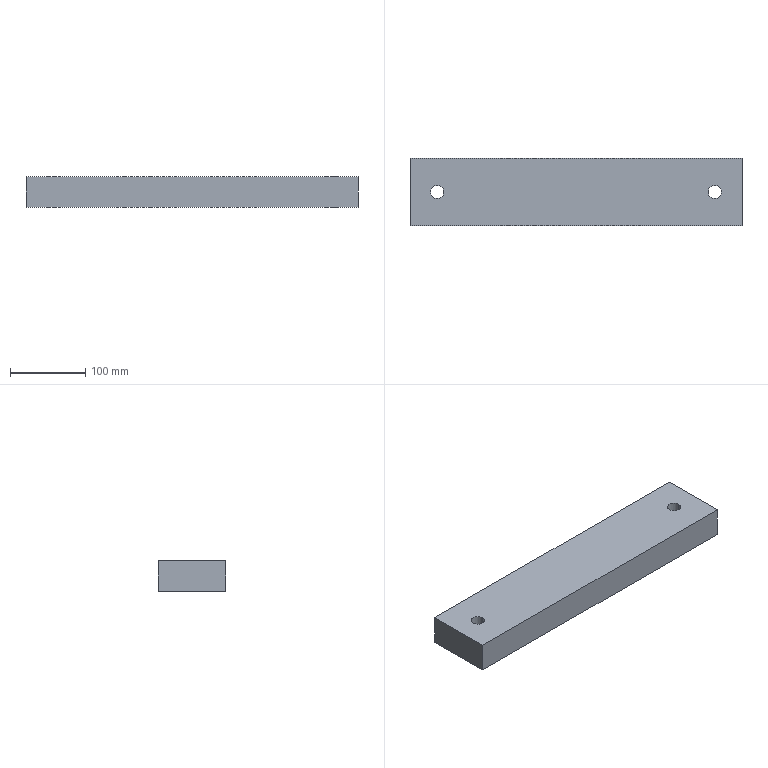Part | SolidWorks | features Extrusion 1, HoleWzd 1 | 1 solid | 10 faces | box 440 x 90 x 40 mm | volume 1564758 mm3 | plane 6 | cylinder 4 | commonest cylinder face diameters 17.5 x4
STEP:
#1=CARTESIAN_POINT('',(27.25,45.,0.));
#2=VERTEX_POINT('',#1);
#3=CARTESIAN_POINT('',(44.75,45.,0.));
#4=VERTEX_POINT('',#3);
#5=CARTESIAN_POINT('',(36.,45.,0.));
#6=DIRECTION('',(0.,0.,1.));
#7=DIRECTION('',(1.,0.,0.));
#8=AXIS2_PLACEMENT_3D('',#5,#6,#7);
#9=CIRCLE('',#8,8.75);
#10=EDGE_CURVE('',#2,#4,#9,.T.);
#11=ORIENTED_EDGE('',*,*,#10,.F.);
#12=CARTESIAN_POINT('',(27.25,45.,40.));
#13=VERTEX_POINT('',#12);
#14=CARTESIAN_POINT('',(27.25,45.,40.));
#15=DIRECTION('',(0.,0.,1.));
#16=VECTOR('',#15,1000.);
#17=LINE('',#14,#16);
#18=EDGE_CURVE('',#2,#13,#17,.T.);
#19=ORIENTED_EDGE('',*,*,#18,.T.);
#20=CARTESIAN_POINT('',(44.75,45.,40.));
#21=VERTEX_POINT('',#20);
#22=CARTESIAN_POINT('',(36.,45.,40.));
#23=DIRECTION('',(0.,0.,1.));
#24=DIRECTION('',(1.,0.,0.));
#25=AXIS2_PLACEMENT_3D('',#22,#23,#24);
#26=CIRCLE('',#25,8.75);
#27=EDGE_CURVE('',#13,#21,#26,.T.);
#28=ORIENTED_EDGE('',*,*,#27,.T.);
#29=CARTESIAN_POINT('',(44.75,45.,40.));
#30=DIRECTION('',(0.,0.,1.));
#31=VECTOR('',#30,1000.);
#32=LINE('',#29,#31);
#33=EDGE_CURVE('',#4,#21,#32,.T.);
#34=ORIENTED_EDGE('',*,*,#33,.F.);
#35=EDGE_LOOP('',(#11,#19,#28,#34));
#36=FACE_OUTER_BOUND('',#35,.T.);
#37=CARTESIAN_POINT('',(36.,45.,40.));
#38=DIRECTION('',(0.,0.,1.));
#39=DIRECTION('',(1.,0.,0.));
#40=AXIS2_PLACEMENT_3D('',#37,#38,#39);
#41=CYLINDRICAL_SURFACE('',#40,8.75);
#42=ADVANCED_FACE('',(#36),#41,.F.);
#43=CARTESIAN_POINT('',(395.25,45.,0.));
#44=VERTEX_POINT('',#43);
#45=CARTESIAN_POINT('',(412.75,45.,0.));
#46=VERTEX_POINT('',#45);
#47=CARTESIAN_POINT('',(404.,45.,0.));
#48=DIRECTION('',(0.,0.,1.));
#49=DIRECTION('',(1.,0.,0.));
#50=AXIS2_PLACEMENT_3D('',#47,#48,#49);
#51=CIRCLE('',#50,8.75);
#52=EDGE_CURVE('',#44,#46,#51,.T.);
#53=ORIENTED_EDGE('',*,*,#52,.F.);
#54=CARTESIAN_POINT('',(395.25,45.,40.));
#55=VERTEX_POINT('',#54);
#56=CARTESIAN_POINT('',(395.25,45.,40.));
#57=DIRECTION('',(0.,0.,1.));
#58=VECTOR('',#57,1000.);
#59=LINE('',#56,#58);
#60=EDGE_CURVE('',#44,#55,#59,.T.);
#61=ORIENTED_EDGE('',*,*,#60,.T.);
#62=CARTESIAN_POINT('',(412.75,45.,40.));
#63=VERTEX_POINT('',#62);
#64=CARTESIAN_POINT('',(404.,45.,40.));
#65=DIRECTION('',(0.,0.,1.));
#66=DIRECTION('',(1.,0.,0.));
#67=AXIS2_PLACEMENT_3D('',#64,#65,#66);
#68=CIRCLE('',#67,8.75);
#69=EDGE_CURVE('',#55,#63,#68,.T.);
#70=ORIENTED_EDGE('',*,*,#69,.T.);
#71=CARTESIAN_POINT('',(412.75,45.,40.));
#72=DIRECTION('',(0.,0.,1.));
#73=VECTOR('',#72,1000.);
#74=LINE('',#71,#73);
#75=EDGE_CURVE('',#46,#63,#74,.T.);
#76=ORIENTED_EDGE('',*,*,#75,.F.);
#77=EDGE_LOOP('',(#53,#61,#70,#76));
#78=FACE_OUTER_BOUND('',#77,.T.);
#79=CARTESIAN_POINT('',(404.,45.,40.));
#80=DIRECTION('',(0.,0.,1.));
#81=DIRECTION('',(1.,0.,0.));
#82=AXIS2_PLACEMENT_3D('',#79,#80,#81);
#83=CYLINDRICAL_SURFACE('',#82,8.75);
#84=ADVANCED_FACE('',(#78),#83,.F.);
#85=CARTESIAN_POINT('',(0.,90.,0.));
#86=VERTEX_POINT('',#85);
#87=CARTESIAN_POINT('',(0.,0.,0.));
#88=VERTEX_POINT('',#87);
#89=CARTESIAN_POINT('',(0.,0.,0.));
#90=DIRECTION('',(0.,-1.,0.));
#91=VECTOR('',#90,1000.);
#92=LINE('',#89,#91);
#93=EDGE_CURVE('',#86,#88,#92,.T.);
#94=ORIENTED_EDGE('',*,*,#93,.T.);
#95=CARTESIAN_POINT('',(0.,0.,40.));
#96=VERTEX_POINT('',#95);
#97=CARTESIAN_POINT('',(0.,0.,40.));
#98=DIRECTION('',(0.,0.,-1.));
#99=VECTOR('',#98,1000.);
#100=LINE('',#97,#99);
#101=EDGE_CURVE('',#96,#88,#100,.T.);
#102=ORIENTED_EDGE('',*,*,#101,.F.);
#103=CARTESIAN_POINT('',(0.,90.,40.));
#104=VERTEX_POINT('',#103);
#105=CARTESIAN_POINT('',(0.,0.,40.));
#106=DIRECTION('',(0.,-1.,0.));
#107=VECTOR('',#106,1000.);
#108=LINE('',#105,#107);
#109=EDGE_CURVE('',#104,#96,#108,.T.);
#110=ORIENTED_EDGE('',*,*,#109,.F.);
#111=CARTESIAN_POINT('',(0.,90.,40.));
#112=DIRECTION('',(0.,0.,-1.));
#113=VECTOR('',#112,1000.);
#114=LINE('',#111,#113);
#115=EDGE_CURVE('',#104,#86,#114,.T.);
#116=ORIENTED_EDGE('',*,*,#115,.T.);
#117=EDGE_LOOP('',(#94,#102,#110,#116));
#118=FACE_OUTER_BOUND('',#117,.T.);
#119=CARTESIAN_POINT('',(0.,0.,40.));
#120=DIRECTION('',(1.,0.,0.));
#121=DIRECTION('',(0.,0.,-1.));
#122=AXIS2_PLACEMENT_3D('',#119,#120,#121);
#123=PLANE('',#122);
#124=ADVANCED_FACE('',(#118),#123,.F.);
#125=CARTESIAN_POINT('',(440.,0.,0.));
#126=VERTEX_POINT('',#125);
#127=CARTESIAN_POINT('',(0.,0.,0.));
#128=DIRECTION('',(1.,0.,0.));
#129=VECTOR('',#128,1000.);
#130=LINE('',#127,#129);
#131=EDGE_CURVE('',#88,#126,#130,.T.);
#132=ORIENTED_EDGE('',*,*,#131,.T.);
#133=CARTESIAN_POINT('',(440.,0.,40.));
#134=VERTEX_POINT('',#133);
#135=CARTESIAN_POINT('',(440.,0.,40.));
#136=DIRECTION('',(0.,0.,-1.));
#137=VECTOR('',#136,1000.);
#138=LINE('',#135,#137);
#139=EDGE_CURVE('',#134,#126,#138,.T.);
#140=ORIENTED_EDGE('',*,*,#139,.F.);
#141=CARTESIAN_POINT('',(0.,0.,40.));
#142=DIRECTION('',(1.,0.,0.));
#143=VECTOR('',#142,1000.);
#144=LINE('',#141,#143);
#145=EDGE_CURVE('',#96,#134,#144,.T.);
#146=ORIENTED_EDGE('',*,*,#145,.F.);
#147=ORIENTED_EDGE('',*,*,#101,.T.);
#148=EDGE_LOOP('',(#132,#140,#146,#147));
#149=FACE_OUTER_BOUND('',#148,.T.);
#150=CARTESIAN_POINT('',(0.,0.,40.));
#151=DIRECTION('',(0.,1.,0.));
#152=DIRECTION('',(0.,0.,1.));
#153=AXIS2_PLACEMENT_3D('',#150,#151,#152);
#154=PLANE('',#153);
#155=ADVANCED_FACE('',(#149),#154,.F.);
#156=CARTESIAN_POINT('',(440.,90.,0.));
#157=VERTEX_POINT('',#156);
#158=CARTESIAN_POINT('',(440.,0.,0.));
#159=DIRECTION('',(0.,1.,0.));
#160=VECTOR('',#159,1000.);
#161=LINE('',#158,#160);
#162=EDGE_CURVE('',#126,#157,#161,.T.);
#163=ORIENTED_EDGE('',*,*,#162,.T.);
#164=CARTESIAN_POINT('',(440.,90.,40.));
#165=VERTEX_POINT('',#164);
#166=CARTESIAN_POINT('',(440.,90.,40.));
#167=DIRECTION('',(0.,0.,-1.));
#168=VECTOR('',#167,1000.);
#169=LINE('',#166,#168);
#170=EDGE_CURVE('',#165,#157,#169,.T.);
#171=ORIENTED_EDGE('',*,*,#170,.F.);
#172=CARTESIAN_POINT('',(440.,0.,40.));
#173=DIRECTION('',(0.,1.,0.));
#174=VECTOR('',#173,1000.);
#175=LINE('',#172,#174);
#176=EDGE_CURVE('',#134,#165,#175,.T.);
#177=ORIENTED_EDGE('',*,*,#176,.F.);
#178=ORIENTED_EDGE('',*,*,#139,.T.);
#179=EDGE_LOOP('',(#163,#171,#177,#178));
#180=FACE_OUTER_BOUND('',#179,.T.);
#181=CARTESIAN_POINT('',(440.,0.,40.));
#182=DIRECTION('',(-1.,0.,0.));
#183=DIRECTION('',(0.,0.,1.));
#184=AXIS2_PLACEMENT_3D('',#181,#182,#183);
#185=PLANE('',#184);
#186=ADVANCED_FACE('',(#180),#185,.F.);
#187=CARTESIAN_POINT('',(0.,90.,0.));
#188=DIRECTION('',(-1.,0.,0.));
#189=VECTOR('',#188,1000.);
#190=LINE('',#187,#189);
#191=EDGE_CURVE('',#157,#86,#190,.T.);
#192=ORIENTED_EDGE('',*,*,#191,.T.);
#193=ORIENTED_EDGE('',*,*,#115,.F.);
#194=CARTESIAN_POINT('',(0.,90.,40.));
#195=DIRECTION('',(-1.,0.,0.));
#196=VECTOR('',#195,1000.);
#197=LINE('',#194,#196);
#198=EDGE_CURVE('',#165,#104,#197,.T.);
#199=ORIENTED_EDGE('',*,*,#198,.F.);
#200=ORIENTED_EDGE('',*,*,#170,.T.);
#201=EDGE_LOOP('',(#192,#193,#199,#200));
#202=FACE_OUTER_BOUND('',#201,.T.);
#203=CARTESIAN_POINT('',(0.,90.,40.));
#204=DIRECTION('',(0.,-1.,0.));
#205=DIRECTION('',(0.,0.,-1.));
#206=AXIS2_PLACEMENT_3D('',#203,#204,#205);
#207=PLANE('',#206);
#208=ADVANCED_FACE('',(#202),#207,.F.);
#209=CARTESIAN_POINT('',(36.,45.,40.));
#210=DIRECTION('',(0.,0.,1.));
#211=DIRECTION('',(1.,0.,0.));
#212=AXIS2_PLACEMENT_3D('',#209,#210,#211);
#213=CIRCLE('',#212,8.75);
#214=EDGE_CURVE('',#21,#13,#213,.T.);
#215=ORIENTED_EDGE('',*,*,#214,.F.);
#216=ORIENTED_EDGE('',*,*,#27,.F.);
#217=EDGE_LOOP('',(#215,#216));
#218=FACE_BOUND('',#217,.T.);
#219=CARTESIAN_POINT('',(404.,45.,40.));
#220=DIRECTION('',(0.,0.,1.));
#221=DIRECTION('',(1.,0.,0.));
#222=AXIS2_PLACEMENT_3D('',#219,#220,#221);
#223=CIRCLE('',#222,8.75);
#224=EDGE_CURVE('',#63,#55,#223,.T.);
#225=ORIENTED_EDGE('',*,*,#224,.F.);
#226=ORIENTED_EDGE('',*,*,#69,.F.);
#227=EDGE_LOOP('',(#225,#226));
#228=FACE_BOUND('',#227,.T.);
#229=ORIENTED_EDGE('',*,*,#109,.T.);
#230=ORIENTED_EDGE('',*,*,#145,.T.);
#231=ORIENTED_EDGE('',*,*,#176,.T.);
#232=ORIENTED_EDGE('',*,*,#198,.T.);
#233=EDGE_LOOP('',(#229,#230,#231,#232));
#234=FACE_OUTER_BOUND('',#233,.T.);
#235=CARTESIAN_POINT('',(0.,90.,40.));
#236=DIRECTION('',(0.,0.,-1.));
#237=DIRECTION('',(-1.,0.,0.));
#238=AXIS2_PLACEMENT_3D('',#235,#236,#237);
#239=PLANE('',#238);
#240=ADVANCED_FACE('',(#218,#228,#234),#239,.F.);
#241=CARTESIAN_POINT('',(36.,45.,0.));
#242=DIRECTION('',(0.,0.,1.));
#243=DIRECTION('',(1.,0.,0.));
#244=AXIS2_PLACEMENT_3D('',#241,#242,#243);
#245=CIRCLE('',#244,8.75);
#246=EDGE_CURVE('',#4,#2,#245,.T.);
#247=ORIENTED_EDGE('',*,*,#246,.T.);
#248=ORIENTED_EDGE('',*,*,#10,.T.);
#249=EDGE_LOOP('',(#247,#248));
#250=FACE_BOUND('',#249,.T.);
#251=CARTESIAN_POINT('',(404.,45.,0.));
#252=DIRECTION('',(0.,0.,1.));
#253=DIRECTION('',(1.,0.,0.));
#254=AXIS2_PLACEMENT_3D('',#251,#252,#253);
#255=CIRCLE('',#254,8.75);
#256=EDGE_CURVE('',#46,#44,#255,.T.);
#257=ORIENTED_EDGE('',*,*,#256,.T.);
#258=ORIENTED_EDGE('',*,*,#52,.T.);
#259=EDGE_LOOP('',(#257,#258));
#260=FACE_BOUND('',#259,.T.);
#261=ORIENTED_EDGE('',*,*,#93,.F.);
#262=ORIENTED_EDGE('',*,*,#191,.F.);
#263=ORIENTED_EDGE('',*,*,#162,.F.);
#264=ORIENTED_EDGE('',*,*,#131,.F.);
#265=EDGE_LOOP('',(#261,#262,#263,#264));
#266=FACE_OUTER_BOUND('',#265,.T.);
#267=CARTESIAN_POINT('',(0.,90.,0.));
#268=DIRECTION('',(0.,0.,-1.));
#269=DIRECTION('',(-1.,0.,0.));
#270=AXIS2_PLACEMENT_3D('',#267,#268,#269);
#271=PLANE('',#270);
#272=ADVANCED_FACE('',(#250,#260,#266),#271,.T.);
#273=ORIENTED_EDGE('',*,*,#60,.F.);
#274=ORIENTED_EDGE('',*,*,#256,.F.);
#275=ORIENTED_EDGE('',*,*,#75,.T.);
#276=ORIENTED_EDGE('',*,*,#224,.T.);
#277=EDGE_LOOP('',(#273,#274,#275,#276));
#278=FACE_OUTER_BOUND('',#277,.T.);
#279=CARTESIAN_POINT('',(404.,45.,40.));
#280=DIRECTION('',(0.,0.,1.));
#281=DIRECTION('',(1.,0.,0.));
#282=AXIS2_PLACEMENT_3D('',#279,#280,#281);
#283=CYLINDRICAL_SURFACE('',#282,8.75);
#284=ADVANCED_FACE('',(#278),#283,.F.);
#285=ORIENTED_EDGE('',*,*,#18,.F.);
#286=ORIENTED_EDGE('',*,*,#246,.F.);
#287=ORIENTED_EDGE('',*,*,#33,.T.);
#288=ORIENTED_EDGE('',*,*,#214,.T.);
#289=EDGE_LOOP('',(#285,#286,#287,#288));
#290=FACE_OUTER_BOUND('',#289,.T.);
#291=CARTESIAN_POINT('',(36.,45.,40.));
#292=DIRECTION('',(0.,0.,1.));
#293=DIRECTION('',(1.,0.,0.));
#294=AXIS2_PLACEMENT_3D('',#291,#292,#293);
#295=CYLINDRICAL_SURFACE('',#294,8.75);
#296=ADVANCED_FACE('',(#290),#295,.F.);
#297=CLOSED_SHELL('',(#42,#84,#124,#155,#186,#208,#240,#272,#284,#296));
#298=MANIFOLD_SOLID_BREP('',#297);
#299=CARTESIAN_POINT('',(0.,0.,0.));
#300=DIRECTION('',(0.,0.,1.));
#301=DIRECTION('',(1.,0.,0.));
#302=AXIS2_PLACEMENT_3D('',#299,#300,#301);
#303=(LENGTH_UNIT()NAMED_UNIT(*)SI_UNIT(.MILLI.,.METRE.));
#304=UNCERTAINTY_MEASURE_WITH_UNIT(LENGTH_MEASURE(0.00001),#303,'','');
#305=(NAMED_UNIT(*)PLANE_ANGLE_UNIT()SI_UNIT($,.RADIAN.));
#306=(NAMED_UNIT(*)SI_UNIT($,.STERADIAN.)SOLID_ANGLE_UNIT());
#307=(GEOMETRIC_REPRESENTATION_CONTEXT(3)GLOBAL_UNCERTAINTY_ASSIGNED_CONTEXT((#304))GLOBAL_UNIT_ASSIGNED_CONTEXT((#303,#305,#306))REPRESENTATION_CONTEXT('',''));
#308=ADVANCED_BREP_SHAPE_REPRESENTATION('',(#298,#302),#307);